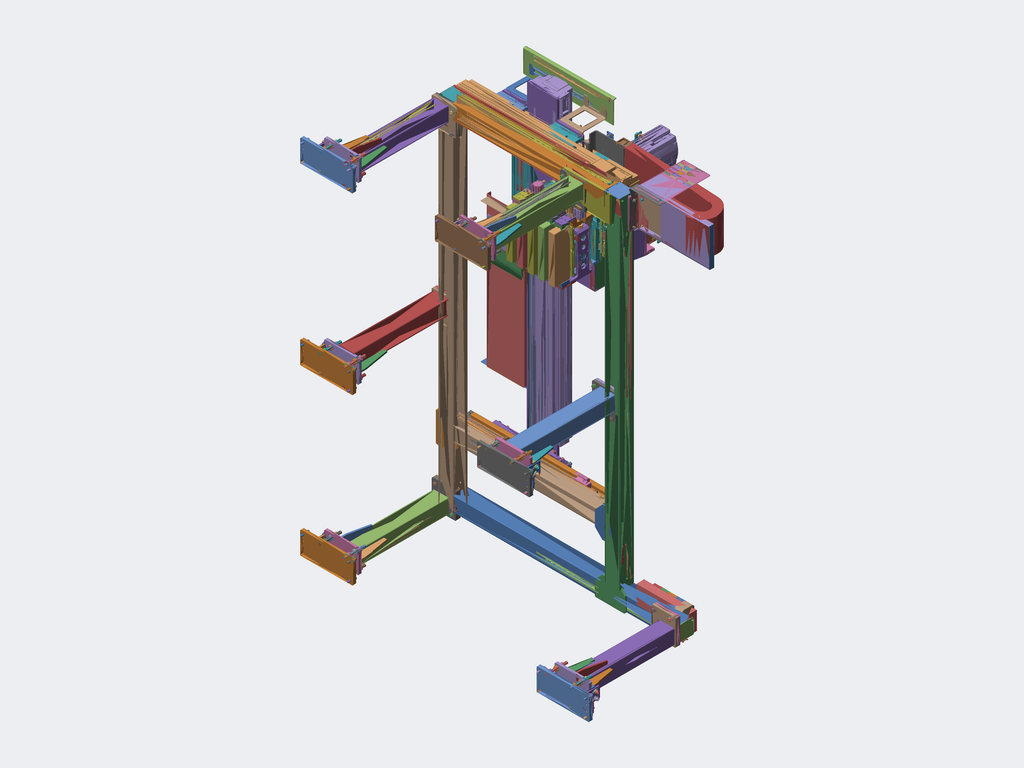Assembly | STEP file | 3599 different items | 3599 placed
Parts list (item | name | quantity | parent item | size | volume), first 284 of 3599 items:
1 | [LR-XN11P]-Part-1 | x1 | in [LR-XN11P] | 12.6 x 34.5 x 105.605 mm | 23912 mm3
2 | [LR-XN11P]-Part-2 | x1 | in [LR-XN11P] | 2.25 x 17.6 x 14.4 mm | 152.141 mm3
3 | [LR-XN12P]-Part-1 | x1 | in [LR-XN12P] | 14.78 x 34.5 x 105.605 mm | 23972 mm3
4 | [LR-XN12P]-Part-2 | x1 | in [LR-XN12P] | 2.25 x 17.6 x 14.4 mm | 152.141 mm3
5 | [LR-XN12P]-Part-1-1 | x1 | in [LR-XN12P]-1 | 14.78 x 34.5 x 105.605 mm | 23972 mm3
6 | [LR-XN12P]-Part-2-1 | x1 | in [LR-XN12P]-1 | 2.25 x 17.6 x 14.4 mm | 152.141 mm3
7 | [LR-XN12P]-Part-1-2 | x1 | in [LR-XN12P]-2 | 14.78 x 34.5 x 105.605 mm | 23972 mm3
8 | [LR-XN12P]-Part-2-2 | x1 | in [LR-XN12P]-2 | 2.25 x 17.6 x 14.4 mm | 152.141 mm3
9 | [LR-XN12P]-Part-1-3 | x1 | in [LR-XN12P]-3 | 14.78 x 34.5 x 105.605 mm | 23972 mm3
10 | [LR-XN12P]-Part-2-3 | x1 | in [LR-XN12P]-3 | 2.25 x 17.6 x 14.4 mm | 152.141 mm3
11 | [OP-26751]-Part-1 | x1 | in [OP-26751] | 6 x 53.8 x 20.8 mm | 4707 mm3
12 | [OP-26751]-Part-2 | x1 | in [OP-26751] | 6 x 53.8 x 20.8 mm | 4707 mm3
13 | SANBN6-25-Part-1 | x1 | in SANBN6-25 | 25 x 6 x 6 mm | 665.544 mm3
14 | SANBN6-25-Part-2 | x1 | in SANBN6-25 | 4 x 10 x 11.5 mm | 231.302 mm3
15 | SANBN6-25-Part-1-1 | x1 | in SANBN6-25-1 | 25 x 6 x 6 mm | 665.544 mm3
16 | SANBN6-25-Part-2-1 | x1 | in SANBN6-25-1 | 4 x 10 x 11.5 mm | 231.302 mm3
17 | SANBN6-25-Part-1-2 | x1 | in SANBN6-25-2 | 25 x 6 x 6 mm | 665.544 mm3
18 | SANBN6-25-Part-2-2 | x1 | in SANBN6-25-2 | 4 x 10 x 11.5 mm | 231.302 mm3
19 | SANBN6-25-Part-1-3 | x1 | in SANBN6-25-3 | 25 x 6 x 6 mm | 665.544 mm3
20 | SANBN6-25-Part-2-3 | x1 | in SANBN6-25-3 | 4 x 10 x 11.5 mm | 231.302 mm3
21 | 25A-CDQ2B40-45DZ-M9BWSDPC-Part-1 | x1 | in 25A-CDQ2B40-45DZ-M9BWSDPC | 84.5 x 52 x 57 mm | 122749 mm3
22 | 25A-CDQ2B40-45DZ-M9BWSDPC-Part-2 | x1 | in 25A-CDQ2B40-45DZ-M9BWSDPC | 27 x 4 x 4.6 mm | 354.995 mm3
23 | 25A-CDQ2B40-45DZ-M9BWSDPC-Part-3 | x1 | in 25A-CDQ2B40-45DZ-M9BWSDPC | 27 x 4 x 4.6 mm | 354.995 mm3
24 | 25A-CDQ2B40-45DZ-M9BWSDPC-Part-1-1 | x1 | in 25A-CDQ2B40-45DZ-M9BWSDPC-1 | 27 x 4 x 4.6 mm | 354.995 mm3
25 | 25A-CDQ2B40-45DZ-M9BWSDPC-Part-2-1 | x1 | in 25A-CDQ2B40-45DZ-M9BWSDPC-1 | 27 x 4 x 4.6 mm | 354.995 mm3
26 | 25A-CDQ2B40-45DZ-M9BWSDPC-Part-3-1 | x1 | in 25A-CDQ2B40-45DZ-M9BWSDPC-1 | 84.5 x 52 x 57 mm | 122749 mm3
27 | J454-EBZ05-98-04-Part-1 | x1 | in J454-EBZ05-98-04 | 380 x 13 x 15 mm | 62425 mm3
28 | J454-EBZ05-98-04-Part-1-1 | x1 | in J454-EBZ05-98-04-1 | 380 x 13 x 15 mm | 62425 mm3
29 | AS2201FG-01-06S | x1 | in Unit 4 purchased part 1 | 14.2 x 35.2 x 27.5 mm | 4200 mm3
30 | AS2201FG-01-06S-1 | x1 | in Unit 4 purchased part 1 | 14.2 x 35.2 x 27.5 mm | 4200 mm3
31 | AS2201FG-01-06S-2 | x1 | in Unit 4 purchased part 1 | 14.2 x 35.2 x 27.5 mm | 4200 mm3
32 | AS2201FG-01-06S-3 | x1 | in Unit 4 purchased part 1 | 14.2 x 35.2 x 27.5 mm | 4200 mm3
33 | AS2002FG-06A | x1 | in Unit 4 purchased part 1 | 12.3 x 31.4 x 43.1 mm | 6190 mm3
34 | AS2002FG-06A-1 | x1 | in Unit 4 purchased part 1 | 12.3 x 31.4 x 43.1 mm | 6190 mm3
35 | AS2002FG-06A-2 | x1 | in Unit 4 purchased part 1 | 12.3 x 31.4 x 43.1 mm | 6190 mm3
36 | AS2002FG-06A-3 | x1 | in Unit 4 purchased part 1 | 12.3 x 31.4 x 43.1 mm | 6190 mm3
37 | AS2002FG-06A-4 | x1 | in Unit 4 purchased part 1 | 12.3 x 31.4 x 43.1 mm | 6190 mm3
38 | AS2002FG-06A-5 | x1 | in Unit 4 purchased part 1 | 12.3 x 31.4 x 43.1 mm | 6190 mm3
39 | AS2002FG-06A-6 | x1 | in Unit 4 purchased part 1 | 12.3 x 31.4 x 43.1 mm | 6190 mm3
40 | AS2002FG-06A-7 | x1 | in Unit 4 purchased part 1 | 12.3 x 31.4 x 43.1 mm | 6190 mm3
41 | AS2002FG-06A-8 | x1 | in Unit 4 purchased part 1 | 12.3 x 31.4 x 43.1 mm | 6190 mm3
42 | AS2002FG-06A-9 | x1 | in Unit 4 purchased part 1 | 12.3 x 31.4 x 43.1 mm | 6190 mm3
43 | BB62-M3-30L | x1 | in Unit 4 purchased part 1 | 5.5 x 33 x 5.5 mm | 272.045 mm3
44 | BB62-M3-30L-1 | x1 | in Unit 4 purchased part 1 | 5.5 x 33 x 5.5 mm | 272.045 mm3
45 | BB62-M3-30L-2 | x1 | in Unit 4 purchased part 1 | 5.5 x 33 x 5.5 mm | 272.045 mm3
46 | BB62-M3-30L-3 | x1 | in Unit 4 purchased part 1 | 5.5 x 33 x 5.5 mm | 272.045 mm3
47 | BB62-M3-30L-4 | x1 | in Unit 4 purchased part 1 | 5.5 x 33 x 5.5 mm | 272.045 mm3
48 | BB62-M3-30L-5 | x1 | in Unit 4 purchased part 1 | 5.5 x 33 x 5.5 mm | 272.045 mm3
49 | BB62-M3-30L-6 | x1 | in Unit 4 purchased part 1 | 5.5 x 33 x 5.5 mm | 272.045 mm3
50 | BB62-M3-30L-7 | x1 | in Unit 4 purchased part 1 | 5.5 x 33 x 5.5 mm | 272.045 mm3
51 | J454-EBZ05-06-00-Part-1 | x1 | in J454-EBZ05-06-00 | 406 x 216 x 12.5 mm | 586432 mm3
52 | BB62-M5-12L | x1 | in J454-EBZ05-06-00 | 8.5 x 17 x 8.5 mm | 467.118 mm3
53 | BB62-M5-12L-1 | x1 | in J454-EBZ05-06-00 | 8.5 x 17 x 8.5 mm | 467.118 mm3
54 | BB62-M5-12L-2 | x1 | in J454-EBZ05-06-00 | 8.5 x 17 x 8.5 mm | 467.118 mm3
55 | BB62-M5-12L-3 | x1 | in J454-EBZ05-06-00 | 8.5 x 17 x 8.5 mm | 467.118 mm3
56 | BB62-M5-12L-4 | x1 | in J454-EBZ05-06-00 | 8.5 x 17 x 8.5 mm | 467.118 mm3
57 | BB62-M5-12L-5 | x1 | in J454-EBZ05-06-00 | 8.5 x 17 x 8.5 mm | 467.118 mm3
58 | BB62-M5-12L-6 | x1 | in J454-EBZ05-06-00 | 8.5 x 17 x 8.5 mm | 467.118 mm3
59 | BB62-M5-12L-7 | x1 | in J454-EBZ05-06-00 | 8.5 x 17 x 8.5 mm | 467.118 mm3
60 | ZZ21-M5 | x1 | in J454-EBZ05-06-00 | 12 x 0.8 x 12 mm | 71.471 mm3
61 | ZZ24-M5 | x1 | in J454-EBZ05-06-00 | 9.2 x 1.3 x 9.188 mm | 56.371 mm3
62 | BB62-M5-20L | x1 | in J454-EBZ05-06-00 | 8.5 x 25 x 8.5 mm | 624.198 mm3
63 | ZZ24-M5-1 | x1 | in J454-EBZ05-06-00 | 9.2 x 1.3 x 9.188 mm | 56.371 mm3
64 | ZZ21-M5-1 | x1 | in J454-EBZ05-06-00 | 12 x 0.8 x 12 mm | 71.471 mm3
65 | BB62-M5-20L-1 | x1 | in J454-EBZ05-06-00 | 8.5 x 25 x 8.5 mm | 624.198 mm3
66 | ZZ24-M5-2 | x1 | in J454-EBZ05-06-00 | 9.2 x 1.3 x 9.188 mm | 56.371 mm3
67 | ZZ21-M5-2 | x1 | in J454-EBZ05-06-00 | 12 x 0.8 x 12 mm | 71.471 mm3
68 | BB62-M5-20L-2 | x1 | in J454-EBZ05-06-00 | 8.5 x 25 x 8.5 mm | 624.198 mm3
69 | ZZ24-M5-3 | x1 | in J454-EBZ05-06-00 | 9.2 x 1.3 x 9.188 mm | 56.371 mm3
70 | ZZ21-M5-3 | x1 | in J454-EBZ05-06-00 | 12 x 0.8 x 12 mm | 71.471 mm3
71 | BB62-M5-20L-3 | x1 | in J454-EBZ05-06-00 | 8.5 x 25 x 8.5 mm | 624.198 mm3
72 | ZZ24-M5-4 | x1 | in J454-EBZ05-06-00 | 9.2 x 1.3 x 9.188 mm | 56.371 mm3
73 | ZZ21-M5-4 | x1 | in J454-EBZ05-06-00 | 12 x 0.8 x 12 mm | 71.471 mm3
74 | BB62-M5-20L-4 | x1 | in J454-EBZ05-06-00 | 8.5 x 25 x 8.5 mm | 624.198 mm3
75 | ZZ24-M5-5 | x1 | in J454-EBZ05-06-00 | 9.2 x 1.3 x 9.188 mm | 56.371 mm3
76 | ZZ21-M5-5 | x1 | in J454-EBZ05-06-00 | 12 x 0.8 x 12 mm | 71.471 mm3
77 | BB62-M5-20L-5 | x1 | in J454-EBZ05-06-00 | 8.5 x 25 x 8.5 mm | 624.198 mm3
78 | J454-EBZ05-07-00-Part-1 | x1 | in J454-EBZ05-07-00 | 74 x 66 x 38 mm | 56161 mm3
79 | MSTMS8-20 | x1 | in J454-EBZ05-07-00 | 20 x 8 x 7.85 mm | 827.27 mm3
80 | MSTMS8-20-1 | x1 | in J454-EBZ05-07-00 | 20 x 8 x 7.85 mm | 827.27 mm3
81 | BB62-M8-30L | x1 | in J454-EBZ05-07-00 | 13 x 38 x 13 mm | 2381 mm3
82 | BB62-M8-30L-1 | x1 | in J454-EBZ05-07-00 | 13 x 38 x 13 mm | 2381 mm3
83 | ZZ21-M8 | x1 | in J454-EBZ05-07-00 | 18 x 1.6 x 18 mm | 316.358 mm3
84 | ZZ24-M8 | x1 | in J454-EBZ05-07-00 | 15.4 x 2 x 15.4 mm | 263.048 mm3
85 | ZZ21-M8-1 | x1 | in J454-EBZ05-07-00 | 18 x 1.6 x 18 mm | 316.358 mm3
86 | ZZ24-M8-1 | x1 | in J454-EBZ05-07-00 | 15.4 x 2 x 15.4 mm | 263.048 mm3
87 | BB62-M5-90L | x1 | in J454-EBZ05-07-00 | 8.5 x 95 x 8.5 mm | 2008 mm3
88 | BB62-M5-90L-1 | x1 | in J454-EBZ05-07-00 | 8.5 x 95 x 8.5 mm | 2008 mm3
89 | BB62-M5-90L-2 | x1 | in J454-EBZ05-07-00 | 8.5 x 95 x 8.5 mm | 2008 mm3
90 | BB62-M5-90L-3 | x1 | in J454-EBZ05-07-00 | 8.5 x 95 x 8.5 mm | 2008 mm3
91 | J454-EBZ05-05-00-Part-1 | x1 | in J454-EBZ05-05-00 | 180 x 30 x 15 mm | 71858 mm3
92 | MSTMS8-20-2 | x1 | in J454-EBZ05-05-00 | 20 x 8 x 7.85 mm | 856.572 mm3
93 | J454-EBZ05-01-04-Part-1 | x1 | in J454-EBZ05-01-04 | 448 x 200 x 12 mm | 706268 mm3
94 | ZZ21-M8-2 | x1 | in J454-EBZ05-01-04 | 18 x 1.6 x 18 mm | 316.358 mm3
95 | ZZ24-M8-2 | x1 | in J454-EBZ05-01-04 | 15.4 x 2 x 15.383 mm | 252.413 mm3
96 | BB62-M8-65L | x1 | in J454-EBZ05-01-04 | 13 x 73 x 13 mm | 4140 mm3
97 | ZZ24-M8-3 | x1 | in J454-EBZ05-01-04 | 15.4 x 2 x 15.383 mm | 252.413 mm3
98 | ZZ21-M8-3 | x1 | in J454-EBZ05-01-04 | 18 x 1.6 x 18 mm | 316.358 mm3
99 | BB62-M8-65L-1 | x1 | in J454-EBZ05-01-04 | 13 x 73 x 13 mm | 4140 mm3
100 | ZZ24-M8-4 | x1 | in J454-EBZ05-01-04 | 15.4 x 2 x 15.383 mm | 252.413 mm3
101 | ZZ21-M8-4 | x1 | in J454-EBZ05-01-04 | 18 x 1.6 x 18 mm | 316.358 mm3
102 | BB62-M8-65L-2 | x1 | in J454-EBZ05-01-04 | 13 x 73 x 13 mm | 4140 mm3
103 | ZZ24-M8-5 | x1 | in J454-EBZ05-01-04 | 15.4 x 2 x 15.383 mm | 252.413 mm3
104 | ZZ21-M8-5 | x1 | in J454-EBZ05-01-04 | 18 x 1.6 x 18 mm | 316.358 mm3
105 | BB62-M8-65L-3 | x1 | in J454-EBZ05-01-04 | 13 x 73 x 13 mm | 4140 mm3
106 | ZZ24-M8-6 | x1 | in J454-EBZ05-01-04 | 15.4 x 2 x 15.383 mm | 252.413 mm3
107 | ZZ21-M8-6 | x1 | in J454-EBZ05-01-04 | 18 x 1.6 x 18 mm | 316.358 mm3
108 | BB62-M8-65L-4 | x1 | in J454-EBZ05-01-04 | 13 x 73 x 13 mm | 4140 mm3
109 | ZZ24-M8-7 | x1 | in J454-EBZ05-01-04 | 15.4 x 2 x 15.383 mm | 252.413 mm3
110 | ZZ21-M8-7 | x1 | in J454-EBZ05-01-04 | 18 x 1.6 x 18 mm | 316.358 mm3
111 | BB62-M8-65L-5 | x1 | in J454-EBZ05-01-04 | 13 x 73 x 13 mm | 4140 mm3
112 | ZZ24-M8-8 | x1 | in J454-EBZ05-01-04 | 15.4 x 2 x 15.383 mm | 252.413 mm3
113 | ZZ21-M8-8 | x1 | in J454-EBZ05-01-04 | 18 x 1.6 x 18 mm | 316.358 mm3
114 | BB62-M8-65L-6 | x1 | in J454-EBZ05-01-04 | 13 x 73 x 13 mm | 4140 mm3
115 | ZZ24-M8-9 | x1 | in J454-EBZ05-01-04 | 15.4 x 2 x 15.383 mm | 252.413 mm3
116 | ZZ21-M8-9 | x1 | in J454-EBZ05-01-04 | 18 x 1.6 x 18 mm | 316.358 mm3
117 | BB62-M8-65L-7 | x1 | in J454-EBZ05-01-04 | 13 x 73 x 13 mm | 4140 mm3
118 | MSTMS8-20-3 | x1 | in J454-EBZ05-01-04 | 20 x 8 x 7.85 mm | 856.572 mm3
119 | MSTMS8-20-4 | x1 | in J454-EBZ05-01-04 | 20 x 8 x 7.85 mm | 856.572 mm3
120 | BB62-M6-15L | x1 | in J454-EBZ05-01-04 | 10 x 21 x 10 mm | 798.222 mm3
121 | BB62-M6-15L-1 | x1 | in J454-EBZ05-01-04 | 10 x 21 x 10 mm | 798.222 mm3
122 | BB62-M6-15L-2 | x1 | in J454-EBZ05-01-04 | 10 x 21 x 10 mm | 798.222 mm3
123 | BB62-M6-15L-3 | x1 | in J454-EBZ05-01-04 | 10 x 21 x 10 mm | 798.222 mm3
124 | BB62-M6-15L-4 | x1 | in J454-EBZ05-01-04 | 10 x 21 x 10 mm | 798.222 mm3
125 | BB62-M6-15L-5 | x1 | in J454-EBZ05-01-04 | 10 x 21 x 10 mm | 798.222 mm3
126 | BB62-M6-15L-6 | x1 | in J454-EBZ05-01-04 | 10 x 21 x 10 mm | 798.222 mm3
127 | BB62-M6-15L-7 | x1 | in J454-EBZ05-01-04 | 10 x 21 x 10 mm | 798.222 mm3
128 | BB62-M6-15L-8 | x1 | in J454-EBZ05-01-04 | 10 x 21 x 10 mm | 798.222 mm3
129 | BB62-M6-15L-9 | x1 | in J454-EBZ05-01-04 | 10 x 21 x 10 mm | 798.222 mm3
130 | BB62-M6-15L-10 | x1 | in J454-EBZ05-01-04 | 10 x 21 x 10 mm | 798.222 mm3
131 | BB62-M6-15L-11 | x1 | in J454-EBZ05-01-04 | 10 x 21 x 10 mm | 798.222 mm3
132 | MRB-85 | x1 | in J454-EBZ05-01-04 | 85 x 35 x 7.3 mm | 5359 mm3
133 | WSX-SUS-M4X10-1.5 | x1 | in J454-EBZ05-01-04 | 10 x 1.5 x 10 mm | 93.953 mm3
134 | BB62-M4-12L | x1 | in J454-EBZ05-01-04 | 7 x 16 x 7 mm | 280.182 mm3
135 | WSX-SUS-M4X10-1.5-1 | x1 | in J454-EBZ05-01-04 | 10 x 1.5 x 10 mm | 93.953 mm3
136 | BB62-M4-12L-1 | x1 | in J454-EBZ05-01-04 | 7 x 16 x 7 mm | 280.182 mm3
137 | J454-EBZ05-02-00-Part-1 | x1 | in J454-EBZ05-02-00 | 200 x 174 x 12 mm | 291304 mm3
138 | MSTMS8-20-5 | x1 | in J454-EBZ05-02-00 | 20 x 8 x 7.85 mm | 856.572 mm3
139 | MSTMS8-20-6 | x1 | in J454-EBZ05-02-00 | 20 x 8 x 7.85 mm | 856.572 mm3
140 | BB62-M6-15L-12 | x1 | in J454-EBZ05-02-00 | 10 x 21 x 10 mm | 798.222 mm3
141 | BB62-M6-15L-13 | x1 | in J454-EBZ05-02-00 | 10 x 21 x 10 mm | 798.222 mm3
142 | BB62-M6-15L-14 | x1 | in J454-EBZ05-02-00 | 10 x 21 x 10 mm | 798.222 mm3
143 | BB62-M6-15L-15 | x1 | in J454-EBZ05-02-00 | 10 x 21 x 10 mm | 798.222 mm3
144 | BB62-M6-15L-16 | x1 | in J454-EBZ05-02-00 | 10 x 21 x 10 mm | 798.222 mm3
145 | BB62-M6-15L-17 | x1 | in J454-EBZ05-02-00 | 10 x 21 x 10 mm | 798.222 mm3
146 | BB62-M6-15L-18 | x1 | in J454-EBZ05-02-00 | 10 x 21 x 10 mm | 798.222 mm3
147 | BB62-M6-15L-19 | x1 | in J454-EBZ05-02-00 | 10 x 21 x 10 mm | 798.222 mm3
148 | BB62-M6-15L-20 | x1 | in J454-EBZ05-02-00 | 10 x 21 x 10 mm | 798.222 mm3
149 | BB62-M6-15L-21 | x1 | in J454-EBZ05-02-00 | 10 x 21 x 10 mm | 798.222 mm3
150 | MSTMS8-20-7 | x1 | in J454-EBZ05-02-00 | 20 x 8 x 7.85 mm | 856.572 mm3
151 | MSTMS8-20-8 | x1 | in J454-EBZ05-02-00 | 20 x 8 x 7.85 mm | 856.572 mm3
152 | ZZ24-M10 | x1 | in J454-EBZ05-02-00 | 18.4 x 2.5 x 18.378 mm | 434.673 mm3
153 | ZZ24-M10-1 | x1 | in J454-EBZ05-02-00 | 18.4 x 2.5 x 18.378 mm | 434.673 mm3
154 | ZZ24-M10-2 | x1 | in J454-EBZ05-02-00 | 18.4 x 2.5 x 18.378 mm | 434.673 mm3
155 | ZZ24-M10-3 | x1 | in J454-EBZ05-02-00 | 18.4 x 2.5 x 18.378 mm | 434.673 mm3
156 | ZZ24-M10-4 | x1 | in J454-EBZ05-02-00 | 18.4 x 2.5 x 18.378 mm | 434.673 mm3
157 | ZZ24-M10-5 | x1 | in J454-EBZ05-02-00 | 18.4 x 2.5 x 18.378 mm | 434.673 mm3
158 | WSSS20-10-4 | x1 | in J454-EBZ05-02-00 | 4 x 20 x 20 mm | 918.916 mm3
159 | BB62-M10-30L | x1 | in J454-EBZ05-02-00 | 16 x 40 x 16 mm | 3957 mm3
160 | WSSS20-10-4-1 | x1 | in J454-EBZ05-02-00 | 4 x 20 x 20 mm | 918.916 mm3
161 | BB62-M10-30L-1 | x1 | in J454-EBZ05-02-00 | 16 x 40 x 16 mm | 3957 mm3
162 | WSSS20-10-4-2 | x1 | in J454-EBZ05-02-00 | 4 x 20 x 20 mm | 918.916 mm3
163 | BB62-M10-30L-2 | x1 | in J454-EBZ05-02-00 | 16 x 40 x 16 mm | 3957 mm3
164 | WSSS20-10-4-3 | x1 | in J454-EBZ05-02-00 | 4 x 20 x 20 mm | 918.916 mm3
165 | BB62-M10-30L-3 | x1 | in J454-EBZ05-02-00 | 16 x 40 x 16 mm | 3957 mm3
166 | WSSS20-10-4-4 | x1 | in J454-EBZ05-02-00 | 4 x 20 x 20 mm | 918.916 mm3
167 | BB62-M10-30L-4 | x1 | in J454-EBZ05-02-00 | 16 x 40 x 16 mm | 3957 mm3
168 | WSSS20-10-4-5 | x1 | in J454-EBZ05-02-00 | 4 x 20 x 20 mm | 918.916 mm3
169 | BB62-M10-30L-5 | x1 | in J454-EBZ05-02-00 | 16 x 40 x 16 mm | 3957 mm3
170 | J454-EBZ05-04-00-Part-1 | x1 | in J454-EBZ05-04-00 | 87 x 96 x 12 mm | 74063 mm3
171 | ZZ21-M6 | x1 | in J454-EBZ05-04-00 | 13 x 1 x 13 mm | 99.549 mm3
172 | ZZ24-M6 | x1 | in J454-EBZ05-04-00 | 12.2 x 1.5 x 12.188 mm | 124.605 mm3
173 | BB62-M6-25L | x1 | in J454-EBZ05-04-00 | 10 x 31 x 10 mm | 1081 mm3
174 | ZZ24-M6-1 | x1 | in J454-EBZ05-04-00 | 12.2 x 1.5 x 12.188 mm | 124.605 mm3
175 | ZZ21-M6-1 | x1 | in J454-EBZ05-04-00 | 13 x 1 x 13 mm | 99.549 mm3
176 | BB62-M6-25L-1 | x1 | in J454-EBZ05-04-00 | 10 x 31 x 10 mm | 1081 mm3
177 | ZZ24-M6-2 | x1 | in J454-EBZ05-04-00 | 12.2 x 1.5 x 12.188 mm | 124.605 mm3
178 | ZZ21-M6-2 | x1 | in J454-EBZ05-04-00 | 13 x 1 x 13 mm | 99.549 mm3
179 | BB62-M6-25L-2 | x1 | in J454-EBZ05-04-00 | 10 x 31 x 10 mm | 1081 mm3
180 | ZZ24-M6-3 | x1 | in J454-EBZ05-04-00 | 12.2 x 1.5 x 12.188 mm | 124.605 mm3
181 | ZZ21-M6-3 | x1 | in J454-EBZ05-04-00 | 13 x 1 x 13 mm | 99.549 mm3
182 | BB62-M6-25L-3 | x1 | in J454-EBZ05-04-00 | 10 x 31 x 10 mm | 1081 mm3
183 | J454-EBZ05-08-00-Part-1 | x1 | in J454-EBZ05-08-00 | 75 x 92 x 16 mm | 52479 mm3
184 | BB62-M5-90L-4 | x1 | in J454-EBZ05-08-00 | 8.5 x 95 x 8.5 mm | 2008 mm3
185 | BB62-M5-90L-5 | x1 | in J454-EBZ05-08-00 | 8.5 x 95 x 8.5 mm | 2008 mm3
186 | BB62-M5-90L-6 | x1 | in J454-EBZ05-08-00 | 8.5 x 95 x 8.5 mm | 2008 mm3
187 | BB62-M5-90L-7 | x1 | in J454-EBZ05-08-00 | 8.5 x 95 x 8.5 mm | 2008 mm3
188 | MSTMS8-20-9 | x1 | in J454-EBZ05-08-00 | 20 x 8 x 7.85 mm | 827.27 mm3
189 | MSTMS8-20-10 | x1 | in J454-EBZ05-08-00 | 20 x 8 x 7.85 mm | 827.27 mm3
190 | ZZ21-M8-10 | x1 | in J454-EBZ05-08-00 | 18 x 1.6 x 18 mm | 316.358 mm3
191 | ZZ21-M8-11 | x1 | in J454-EBZ05-08-00 | 18 x 1.6 x 18 mm | 316.358 mm3
192 | ZZ24-M8-10 | x1 | in J454-EBZ05-08-00 | 15.4 x 2 x 15.383 mm | 252.413 mm3
193 | ZZ24-M8-11 | x1 | in J454-EBZ05-08-00 | 15.4 x 2 x 15.383 mm | 252.413 mm3
194 | BB62-M8-30L-2 | x1 | in J454-EBZ05-08-00 | 13 x 38 x 13 mm | 2381 mm3
195 | BB62-M8-30L-3 | x1 | in J454-EBZ05-08-00 | 13 x 38 x 13 mm | 2381 mm3
196 | J454-EBZ05-09-00-Part-1 | x1 | in J454-EBZ05-09-00 | 13 x 42 x 16 mm | 7348 mm3
197 | ZZ21-M6-4 | x1 | in J454-EBZ05-09-00 | 13 x 1 x 13 mm | 99.549 mm3
198 | ZZ21-M6-5 | x1 | in J454-EBZ05-09-00 | 13 x 1 x 13 mm | 99.549 mm3
199 | ZZ24-M6-4 | x1 | in J454-EBZ05-09-00 | 12.2 x 1.5 x 12.188 mm | 124.605 mm3
200 | ZZ24-M6-5 | x1 | in J454-EBZ05-09-00 | 12.2 x 1.5 x 12.188 mm | 124.605 mm3
201 | BB62-M6-25L-4 | x1 | in J454-EBZ05-09-00 | 10 x 31 x 10 mm | 1081 mm3
202 | BB62-M6-25L-5 | x1 | in J454-EBZ05-09-00 | 10 x 31 x 10 mm | 1081 mm3
203 | J454-EBZ05-09-00-Part-1-1 | x1 | in J454-EBZ05-09-00-1 | 13 x 42 x 16 mm | 7348 mm3
204 | ZZ21-M6-6 | x1 | in J454-EBZ05-09-00-1 | 13 x 1 x 13 mm | 99.549 mm3
205 | ZZ21-M6-7 | x1 | in J454-EBZ05-09-00-1 | 13 x 1 x 13 mm | 99.549 mm3
206 | ZZ24-M6-6 | x1 | in J454-EBZ05-09-00-1 | 12.2 x 1.5 x 12.188 mm | 124.605 mm3
207 | ZZ24-M6-7 | x1 | in J454-EBZ05-09-00-1 | 12.2 x 1.5 x 12.188 mm | 124.605 mm3
208 | BB62-M6-25L-6 | x1 | in J454-EBZ05-09-00-1 | 10 x 31 x 10 mm | 1081 mm3
209 | BB62-M6-25L-7 | x1 | in J454-EBZ05-09-00-1 | 10 x 31 x 10 mm | 1081 mm3
210 | J454-EBZ05-09-00-Part-1-2 | x1 | in J454-EBZ05-09-00-2 | 13 x 42 x 16 mm | 7348 mm3
211 | ZZ21-M6-8 | x1 | in J454-EBZ05-09-00-2 | 13 x 1 x 13 mm | 99.549 mm3
212 | ZZ21-M6-9 | x1 | in J454-EBZ05-09-00-2 | 13 x 1 x 13 mm | 99.549 mm3
213 | ZZ24-M6-8 | x1 | in J454-EBZ05-09-00-2 | 12.2 x 1.5 x 12.188 mm | 124.605 mm3
214 | ZZ24-M6-9 | x1 | in J454-EBZ05-09-00-2 | 12.2 x 1.5 x 12.188 mm | 124.605 mm3
215 | BB62-M6-25L-8 | x1 | in J454-EBZ05-09-00-2 | 10 x 31 x 10 mm | 1081 mm3
216 | BB62-M6-25L-9 | x1 | in J454-EBZ05-09-00-2 | 10 x 31 x 10 mm | 1081 mm3
217 | J454-EBZ05-09-00-Part-1-3 | x1 | in J454-EBZ05-09-00-3 | 13 x 42 x 16 mm | 7348 mm3
218 | ZZ21-M6-10 | x1 | in J454-EBZ05-09-00-3 | 13 x 1 x 13 mm | 99.549 mm3
219 | ZZ21-M6-11 | x1 | in J454-EBZ05-09-00-3 | 13 x 1 x 13 mm | 99.549 mm3
220 | ZZ24-M6-10 | x1 | in J454-EBZ05-09-00-3 | 12.2 x 1.5 x 12.188 mm | 124.605 mm3
221 | ZZ24-M6-11 | x1 | in J454-EBZ05-09-00-3 | 12.2 x 1.5 x 12.188 mm | 124.605 mm3
222 | BB62-M6-25L-10 | x1 | in J454-EBZ05-09-00-3 | 10 x 31 x 10 mm | 1081 mm3
223 | BB62-M6-25L-11 | x1 | in J454-EBZ05-09-00-3 | 10 x 31 x 10 mm | 1081 mm3
224 | J454-EBZ05-05-00-Part-1-1 | x1 | in J454-EBZ05-05-00-1 | 180 x 30 x 15 mm | 71858 mm3
225 | MSTMS8-20-11 | x1 | in J454-EBZ05-05-00-1 | 20 x 8 x 7.85 mm | 856.572 mm3
226 | J454-EBZ05-32-03 | x1 | in 01_Fixed part | 448 x 120 x 12 mm | 376287 mm3
227 | J454-EBZ05-32-03-1 | x1 | in 01_Fixed part | 448 x 120 x 12 mm | 376287 mm3
228 | 25A-CDQ2B32-15DZ-M9BWSDPC-Part-1 | x1 | in 25A-CDQ2B32-15DZ-M9BWSDPC | 27 x 4 x 4.6 mm | 354.995 mm3
229 | 25A-CDQ2B32-15DZ-M9BWSDPC-Part-2 | x1 | in 25A-CDQ2B32-15DZ-M9BWSDPC | 48 x 45 x 49.5 mm | 58108 mm3
230 | 25A-CDQ2B32-15DZ-M9BWSDPC-Part-3 | x1 | in 25A-CDQ2B32-15DZ-M9BWSDPC | 27 x 4 x 4.6 mm | 354.995 mm3
231 | Rod | x1 | in 25A-CDQ2B32-15DZ-M9BWSDPC | 37 x 32 x 32 mm | 9768 mm3
232 | J454-EBZ05-99-04-Part-1 | x1 | in J454-EBZ05-99-04 | 140 x 16.5 x 20 mm | 40392 mm3
233 | FUF25-70-A | x1 | in Unit 4 purchased part 2-1 | 50 x 25 x 25 mm | 9148 mm3
234 | FUF25-70-A-1 | x1 | in Unit 4 purchased part 2-1 | 50 x 25 x 25 mm | 9148 mm3
235 | FWSSS-D27-V19-T3 | x1 | in Unit 4 purchased part 2-1 | 27 x 27 x 3 mm | 830.951 mm3
236 | FWSSS-D27-V19-T3-1 | x1 | in Unit 4 purchased part 2-1 | 27 x 27 x 3 mm | 830.951 mm3
237 | KQG2H06-01S | x1 | in Unit 4 purchased part 2-1 | 13.856 x 24.3 x 12 mm | 1839 mm3
238 | KQG2H06-01S-1 | x1 | in Unit 4 purchased part 2-1 | 13.856 x 24.3 x 12 mm | 1839 mm3
239 | BB62-M3-40L | x1 | in Unit 4 purchased part 2-1 | 5.5 x 43 x 5.5 mm | 342.731 mm3
240 | BB62-M3-40L-1 | x1 | in Unit 4 purchased part 2-1 | 5.5 x 43 x 5.5 mm | 342.731 mm3
241 | BB62-M5-50L | x1 | in Unit 4 purchased part 2-1 | 8.5 x 55 x 8.5 mm | 1213 mm3
242 | BB62-M5-50L-1 | x1 | in Unit 4 purchased part 2-1 | 8.5 x 55 x 8.5 mm | 1213 mm3
243 | BB62-M5-50L-2 | x1 | in Unit 4 purchased part 2-1 | 8.5 x 55 x 8.5 mm | 1213 mm3
244 | BB62-M5-50L-3 | x1 | in Unit 4 purchased part 2-1 | 8.5 x 55 x 8.5 mm | 1213 mm3
245 | WSSS12-5-3 | x1 | in Unit 4 purchased part 2-1 | 3 x 12 x 12 mm | 278.251 mm3
246 | WSSS12-5-3-1 | x1 | in Unit 4 purchased part 2-1 | 3 x 12 x 12 mm | 278.251 mm3
247 | WSSS12-5-3-2 | x1 | in Unit 4 purchased part 2-1 | 3 x 12 x 12 mm | 278.251 mm3
248 | WSSS12-5-3-3 | x1 | in Unit 4 purchased part 2-1 | 3 x 12 x 12 mm | 278.251 mm3
249 | J454-EBZ05-17-00-Part-1 | x1 | in J454-EBZ05-17-00 | 19 x 19 x 18 mm | 4103 mm3
250 | BB62-M5-15L | x1 | in J454-EBZ05-17-00 | 8.5 x 20 x 8.5 mm | 526.023 mm3
251 | J454-EBZ05-17-00-Part-1-1 | x1 | in J454-EBZ05-17-00-1 | 19 x 19 x 18 mm | 4103 mm3
252 | BB62-M5-15L-1 | x1 | in J454-EBZ05-17-00-1 | 8.5 x 20 x 8.5 mm | 526.023 mm3
253 | LR-XH50-Part-1 | x1 | in LR-XH50 | 9.4 x 39.451 x 29.153 mm | 4011 mm3
254 | WSX-SUS-M5X12-2 | x1 | in J454-EBZ05-18-00 | 12 x 2 x 12 mm | 178.678 mm3
255 | ZZ24-M5-6 | x1 | in J454-EBZ05-18-00 | 9.2 x 1.3 x 9.188 mm | 56.371 mm3
256 | ZZ24-M5-7 | x1 | in J454-EBZ05-18-00 | 9.2 x 1.3 x 9.188 mm | 56.371 mm3
257 | BB62-M5-22L | x1 | in J454-EBZ05-18-00 | 8.5 x 27 x 8.5 mm | 663.468 mm3
258 | BB62-M5-22L-1 | x1 | in J454-EBZ05-18-00 | 8.5 x 27 x 8.5 mm | 663.468 mm3
259 | BB62-M3-8L | x1 | in J454-EBZ05-18-00 | 5.5 x 11 x 5.5 mm | 116.536 mm3
260 | BB62-M3-8L-1 | x1 | in J454-EBZ05-18-00 | 5.5 x 11 x 5.5 mm | 116.536 mm3
261 | WSX-SUS-M5X12-2-1 | x1 | in J454-EBZ05-18-00 | 12 x 2 x 12 mm | 178.678 mm3
262 | J454-EBZ05-13-00-Part-1 | x1 | in J454-EBZ05-13-00 | 200 x 48 x 50 mm | 172584 mm3
263 | BB62-M6-15L-22 | x1 | in J454-EBZ05-13-00 | 10 x 21 x 10 mm | 798.222 mm3
264 | BB62-M6-15L-23 | x1 | in J454-EBZ05-13-00 | 10 x 21 x 10 mm | 798.222 mm3
265 | BB62-M6-15L-24 | x1 | in J454-EBZ05-13-00 | 10 x 21 x 10 mm | 798.222 mm3
266 | SSTBB6-25-Part-1 | x1 | in SSTBB6-25 | 29 x 11.5 x 10 mm | 987.027 mm3
267 | SSTBB6-25-Part-2 | x1 | in SSTBB6-25 | 5 x 11.5 x 10 mm | 290.522 mm3
268 | SSTBB6-25-Part-1-1 | x1 | in SSTBB6-25-1 | 29 x 11.5 x 10 mm | 987.027 mm3
269 | SSTBB6-25-Part-2-1 | x1 | in SSTBB6-25-1 | 5 x 11.5 x 10 mm | 290.522 mm3
270 | SSTBB6-25-Part-1-2 | x1 | in SSTBB6-25-2 | 29 x 11.5 x 10 mm | 987.027 mm3
271 | SSTBB6-25-Part-2-2 | x1 | in SSTBB6-25-2 | 5 x 11.5 x 10 mm | 290.522 mm3
272 | SSTBB6-25-Part-1-3 | x1 | in SSTBB6-25-3 | 29 x 11.5 x 10 mm | 987.027 mm3
273 | SSTBB6-25-Part-2-3 | x1 | in SSTBB6-25-3 | 5 x 11.5 x 10 mm | 290.522 mm3
274 | J454-EBZ05-11-03-Part-1 | x1 | in J454-EBZ05-11-03 | 290 x 48 x 62 mm | 468483 mm3
275 | MSTMS8-20-12 | x1 | in J454-EBZ05-11-03 | 20 x 8 x 7.85 mm | 856.572 mm3
276 | MSTMS8-20-13 | x1 | in J454-EBZ05-11-03 | 20 x 8 x 7.85 mm | 856.572 mm3
277 | BB62-M6-18L | x1 | in J454-EBZ05-11-03 | 10 x 24 x 10 mm | 883.045 mm3
278 | BB62-M6-18L-1 | x1 | in J454-EBZ05-11-03 | 10 x 24 x 10 mm | 883.045 mm3
279 | BB62-M6-18L-2 | x1 | in J454-EBZ05-11-03 | 10 x 24 x 10 mm | 883.045 mm3
280 | BB62-M6-18L-3 | x1 | in J454-EBZ05-11-03 | 10 x 24 x 10 mm | 883.045 mm3
281 | BB62-M6-18L-4 | x1 | in J454-EBZ05-11-03 | 10 x 24 x 10 mm | 883.045 mm3
282 | BB62-M6-18L-5 | x1 | in J454-EBZ05-11-03 | 10 x 24 x 10 mm | 883.045 mm3
283 | KNCLSS3-8-10 | x1 | in J454-EBZ05-11-03 | 10 x 6 x 6 mm | 210.927 mm3
284 | KNCLSS3-8-10-1 | x1 | in J454-EBZ05-11-03 | 10 x 6 x 6 mm | 210.927 mm3
Placements (level | parent | child | x y z in mm | rotation matrix by rows), first 198 of 3891 lines:
1 | subassembly 2 | J454-EBZ05-00-08 | -0.0 1452.0 1475.0 | 0 0 1 0 1 0 -1 0 0
2 | J454-EBZ05-00-08 | 01_Fixed part | -0.0 -0.0 -0.0 | 1 0 0 0 1 0 0 0 1
3 | 01_Fixed part | Unit 4 purchased part 1 | -0.0 -0.0 -0.0 | 1 0 0 0 1 0 0 0 1
4 | Unit 4 purchased part 1 | [LR-XN11P] | 25.945 113.445 -23.2 | -1 0 0 0 0 1 0 1 0
5 | [LR-XN11P] | [LR-XN11P]-Part-1 | -0.0 -0.0 -0.0 | 1 0 0 0 1 0 0 0 1
5 | [LR-XN11P] | [LR-XN11P]-Part-2 | -0.0 -0.0 -0.0 | 1 0 0 0 1 0 0 0 1
4 | Unit 4 purchased part 1 | [LR-XN12P] | 15.245 113.445 -19.0 | -1 0 0 0 0 1 0 1 0
5 | [LR-XN12P] | [LR-XN12P]-Part-1 | -0.0 -0.0 -0.0 | 1 0 0 0 1 0 0 0 1
5 | [LR-XN12P] | [LR-XN12P]-Part-2 | -0.0 -0.0 -0.0 | 1 0 0 0 1 0 0 0 1
4 | Unit 4 purchased part 1 | [LR-XN12P]-1 | 4.545 113.445 -19.0 | -1 0 0 0 0 1 0 1 0
5 | [LR-XN12P]-1 | [LR-XN12P]-Part-1-1 | -0.0 -0.0 -0.0 | 1 0 0 0 1 0 0 0 1
5 | [LR-XN12P]-1 | [LR-XN12P]-Part-2-1 | -0.0 -0.0 -0.0 | 1 0 0 0 1 0 0 0 1
4 | Unit 4 purchased part 1 | [LR-XN12P]-2 | -6.155 113.445 -19.0 | -1 0 0 0 0 1 0 1 0
5 | [LR-XN12P]-2 | [LR-XN12P]-Part-1-2 | -0.0 -0.0 -0.0 | 1 0 0 0 1 0 0 0 1
5 | [LR-XN12P]-2 | [LR-XN12P]-Part-2-2 | -0.0 -0.0 -0.0 | 1 0 0 0 1 0 0 0 1
4 | Unit 4 purchased part 1 | [LR-XN12P]-3 | -16.855 113.445 -19.0 | -1 0 0 0 0 1 0 1 0
5 | [LR-XN12P]-3 | [LR-XN12P]-Part-1-3 | -0.0 -0.0 -0.0 | 1 0 0 0 1 0 0 0 1
5 | [LR-XN12P]-3 | [LR-XN12P]-Part-2-3 | -0.0 -0.0 -0.0 | 1 0 0 0 1 0 0 0 1
4 | Unit 4 purchased part 1 | [OP-26751] | -37.025 181.9 6.75 | 1 0 0 0 -1 0 0 0 -1
5 | [OP-26751] | [OP-26751]-Part-1 | -0.0 -0.0 -0.0 | 1 0 0 0 1 0 0 0 1
5 | [OP-26751] | [OP-26751]-Part-2 | -0.0 -0.0 -0.0 | 1 0 0 0 1 0 0 0 1
4 | Unit 4 purchased part 1 | SANBN6-25 | -115.0 -16.0 205.0 | 0 -0.5 0.866 0 0.866 0.5 -1 0 0
5 | SANBN6-25 | SANBN6-25-Part-1 | -0.0 -0.0 -0.0 | 1 0 0 0 1 0 0 0 1
5 | SANBN6-25 | SANBN6-25-Part-2 | -0.0 -0.0 -0.0 | 1 0 0 0 1 0 0 0 1
4 | Unit 4 purchased part 1 | SANBN6-25-1 | 115.0 -16.0 205.0 | 0 -0.5 0.866 0 0.866 0.5 -1 0 0
5 | SANBN6-25-1 | SANBN6-25-Part-1-1 | -0.0 -0.0 -0.0 | 1 0 0 0 1 0 0 0 1
5 | SANBN6-25-1 | SANBN6-25-Part-2-1 | -0.0 -0.0 -0.0 | 1 0 0 0 1 0 0 0 1
4 | Unit 4 purchased part 1 | SANBN6-25-2 | 115.0 -16.0 -205.0 | 0 0.5 0.866 0 -0.866 0.5 1 0 0
5 | SANBN6-25-2 | SANBN6-25-Part-1-2 | -0.0 -0.0 -0.0 | 1 0 0 0 1 0 0 0 1
5 | SANBN6-25-2 | SANBN6-25-Part-2-2 | -0.0 -0.0 -0.0 | 1 0 0 0 1 0 0 0 1
4 | Unit 4 purchased part 1 | SANBN6-25-3 | -115.0 -16.0 -205.0 | 0 0.5 0.866 0 -0.866 0.5 1 0 0
5 | SANBN6-25-3 | SANBN6-25-Part-1-3 | -0.0 -0.0 -0.0 | 1 0 0 0 1 0 0 0 1
5 | SANBN6-25-3 | SANBN6-25-Part-2-3 | -0.0 -0.0 -0.0 | 1 0 0 0 1 0 0 0 1
4 | Unit 4 purchased part 1 | 25A-CDQ2B40-45DZ-M9BWSDPC | 26.0 -53.0 -291.5 | 0 0 -1 0 1 0 1 0 0
5 | 25A-CDQ2B40-45DZ-M9BWSDPC | 25A-CDQ2B40-45DZ-M9BWSDPC-Part-1 | -0.0 -0.0 -0.0 | 1 0 0 0 1 0 0 0 1
5 | 25A-CDQ2B40-45DZ-M9BWSDPC | 25A-CDQ2B40-45DZ-M9BWSDPC-Part-2 | -0.0 -0.0 -0.0 | 1 0 0 0 1 0 0 0 1
5 | 25A-CDQ2B40-45DZ-M9BWSDPC | 25A-CDQ2B40-45DZ-M9BWSDPC-Part-3 | -0.0 -0.0 -0.0 | 1 0 0 0 1 0 0 0 1
4 | Unit 4 purchased part 1 | 25A-CDQ2B40-45DZ-M9BWSDPC-1 | -26.0 17.0 31.5 | 0 1 0 0 0 1 1 0 0
5 | 25A-CDQ2B40-45DZ-M9BWSDPC-1 | 25A-CDQ2B40-45DZ-M9BWSDPC-Part-1-1 | -0.0 -0.0 -0.0 | 1 0 0 0 1 0 0 0 1
5 | 25A-CDQ2B40-45DZ-M9BWSDPC-1 | 25A-CDQ2B40-45DZ-M9BWSDPC-Part-2-1 | -0.0 -0.0 -0.0 | 1 0 0 0 1 0 0 0 1
5 | 25A-CDQ2B40-45DZ-M9BWSDPC-1 | 25A-CDQ2B40-45DZ-M9BWSDPC-Part-3-1 | -0.0 -0.0 -0.0 | 1 0 0 0 1 0 0 0 1
4 | Unit 4 purchased part 1 | J454-EBZ05-98-04 | 36.5 -10.0 -195.5 | 0 0 1 0 -1 0 1 0 0
5 | J454-EBZ05-98-04 | J454-EBZ05-98-04-Part-1 | -0.0 -0.0 -0.0 | 1 0 0 0 1 0 0 0 1
4 | Unit 4 purchased part 1 | J454-EBZ05-98-04-1 | -83.5 -10.0 -195.5 | 0 0 1 0 -1 0 1 0 0
5 | J454-EBZ05-98-04-1 | J454-EBZ05-98-04-Part-1-1 | -0.0 -0.0 -0.0 | 1 0 0 0 1 0 0 0 1
4 | Unit 4 purchased part 1 | AS2201FG-01-06S | -30.1 -27.0 -284.0 | 0 -1 0 0 0 1 -1 0 0
4 | Unit 4 purchased part 1 | AS2201FG-01-06S-1 | -30.1 -27.0 -219.5 | 0 -1 0 0 0 1 -1 0 0
4 | Unit 4 purchased part 1 | AS2201FG-01-06S-2 | -0.0 73.1 103.5 | 0 0 -1 0 1 0 1 0 0
4 | Unit 4 purchased part 1 | AS2201FG-01-06S-3 | -0.0 73.1 39.0 | 0 0 -1 0 1 0 1 0 0
4 | Unit 4 purchased part 1 | AS2002FG-06A | -168.45 -24.0 -127.4 | -1 0 0 0 0 -1 0 -1 0
4 | Unit 4 purchased part 1 | AS2002FG-06A-1 | -156.15 -24.0 -127.4 | -1 0 0 0 0 -1 0 -1 0
4 | Unit 4 purchased part 1 | AS2002FG-06A-2 | -168.45 -24.0 -83.6 | -1 0 0 0 0 1 0 1 0
4 | Unit 4 purchased part 1 | AS2002FG-06A-3 | -156.15 -24.0 -83.6 | -1 0 0 0 0 1 0 1 0
4 | Unit 4 purchased part 1 | AS2002FG-06A-4 | -168.45 -24.0 7.1 | -1 0 0 0 0 -1 0 -1 0
4 | Unit 4 purchased part 1 | AS2002FG-06A-5 | -156.15 -24.0 7.1 | -1 0 0 0 0 -1 0 -1 0
4 | Unit 4 purchased part 1 | AS2002FG-06A-6 | -168.45 -24.0 83.6 | -1 0 0 0 0 -1 0 -1 0
4 | Unit 4 purchased part 1 | AS2002FG-06A-7 | -156.15 -24.0 83.6 | -1 0 0 0 0 -1 0 -1 0
4 | Unit 4 purchased part 1 | AS2002FG-06A-8 | -168.45 -24.0 127.4 | -1 0 0 0 0 1 0 1 0
4 | Unit 4 purchased part 1 | AS2002FG-06A-9 | -156.15 -24.0 127.4 | -1 0 0 0 0 1 0 1 0
4 | Unit 4 purchased part 1 | BB62-M3-30L | -174.6 -30.3 134.5 | 0 -1 0 0 0 1 -1 0 0
4 | Unit 4 purchased part 1 | BB62-M3-30L-1 | -174.6 -17.7 134.5 | 0 -1 0 0 0 1 -1 0 0
4 | Unit 4 purchased part 1 | BB62-M3-30L-2 | -174.6 -17.7 76.5 | 0 -1 0 0 0 -1 1 0 0
4 | Unit 4 purchased part 1 | BB62-M3-30L-3 | -174.6 -30.3 76.5 | 0 -1 0 0 0 -1 1 0 0
4 | Unit 4 purchased part 1 | BB62-M3-30L-4 | -174.6 -30.3 -76.5 | 0 -1 0 0 0 1 -1 0 0
4 | Unit 4 purchased part 1 | BB62-M3-30L-5 | -174.6 -17.7 -76.5 | 0 -1 0 0 0 1 -1 0 0
4 | Unit 4 purchased part 1 | BB62-M3-30L-6 | -174.6 -17.7 -134.5 | 0 -1 0 0 0 -1 1 0 0
4 | Unit 4 purchased part 1 | BB62-M3-30L-7 | -174.6 -30.3 -134.5 | 0 -1 0 0 0 -1 1 0 0
3 | 01_Fixed part | J454-EBZ05-06-00 | -0.0 -0.0 -0.0 | 0 1 0 0 0 -1 -1 0 0
4 | J454-EBZ05-06-00 | J454-EBZ05-06-00-Part-1 | -0.0 -0.0 -0.0 | 1 0 0 0 1 0 0 0 1
4 | J454-EBZ05-06-00 | BB62-M5-12L | -0.0 -60.0 6.0 | 0 0 1 -1 0 0 0 -1 0
4 | J454-EBZ05-06-00 | BB62-M5-12L-1 | -0.0 60.0 6.0 | 0 0 1 -1 0 0 0 -1 0
4 | J454-EBZ05-06-00 | BB62-M5-12L-2 | -60.0 -60.0 6.0 | 0 0 1 -1 0 0 0 -1 0
4 | J454-EBZ05-06-00 | BB62-M5-12L-3 | -60.0 60.0 6.0 | 0 0 1 -1 0 0 0 -1 0
4 | J454-EBZ05-06-00 | BB62-M5-12L-4 | 60.0 -60.0 6.0 | 0 0 1 -1 0 0 0 -1 0
4 | J454-EBZ05-06-00 | BB62-M5-12L-5 | 60.0 60.0 6.0 | 0 0 1 -1 0 0 0 -1 0
4 | J454-EBZ05-06-00 | BB62-M5-12L-6 | -120.0 60.0 6.0 | 0 0 1 -1 0 0 0 -1 0
4 | J454-EBZ05-06-00 | BB62-M5-12L-7 | -120.0 -60.0 6.0 | 0 0 1 -1 0 0 0 -1 0
4 | J454-EBZ05-06-00 | ZZ21-M5 | -180.0 -60.0 -0.0 | 0 0 -1 1 0 0 0 -1 0
4 | J454-EBZ05-06-00 | ZZ24-M5 | -180.0 -60.0 -0.8 | 0 0 -1 1 0 0 0 -1 0
4 | J454-EBZ05-06-00 | BB62-M5-20L | -180.0 -60.0 -2.1 | 0 0 -1 1 0 0 0 -1 0
4 | J454-EBZ05-06-00 | ZZ24-M5-1 | 120.0 -60.0 -0.8 | 0 0 -1 1 0 0 0 -1 0
4 | J454-EBZ05-06-00 | ZZ21-M5-1 | 120.0 -60.0 -0.0 | 0 0 -1 1 0 0 0 -1 0
4 | J454-EBZ05-06-00 | BB62-M5-20L-1 | 120.0 -60.0 -2.1 | 0 0 -1 1 0 0 0 -1 0
4 | J454-EBZ05-06-00 | ZZ24-M5-2 | 180.0 -60.0 -0.8 | 0 0 -1 1 0 0 0 -1 0
4 | J454-EBZ05-06-00 | ZZ21-M5-2 | 180.0 -60.0 -0.0 | 0 0 -1 1 0 0 0 -1 0
4 | J454-EBZ05-06-00 | BB62-M5-20L-2 | 180.0 -60.0 -2.1 | 0 0 -1 1 0 0 0 -1 0
4 | J454-EBZ05-06-00 | ZZ24-M5-3 | 180.0 60.0 -0.8 | 0 0 -1 1 0 0 0 -1 0
4 | J454-EBZ05-06-00 | ZZ21-M5-3 | 180.0 60.0 -0.0 | 0 0 -1 1 0 0 0 -1 0
4 | J454-EBZ05-06-00 | BB62-M5-20L-3 | 180.0 60.0 -2.1 | 0 0 -1 1 0 0 0 -1 0
4 | J454-EBZ05-06-00 | ZZ24-M5-4 | 120.0 60.0 -0.8 | 0 0 -1 1 0 0 0 -1 0
4 | J454-EBZ05-06-00 | ZZ21-M5-4 | 120.0 60.0 -0.0 | 0 0 -1 1 0 0 0 -1 0
4 | J454-EBZ05-06-00 | BB62-M5-20L-4 | 120.0 60.0 -2.1 | 0 0 -1 1 0 0 0 -1 0
4 | J454-EBZ05-06-00 | ZZ24-M5-5 | -180.0 60.0 -0.8 | 0 0 -1 1 0 0 0 -1 0
4 | J454-EBZ05-06-00 | ZZ21-M5-5 | -180.0 60.0 0.0 | 0 0 -1 1 0 0 0 -1 0
4 | J454-EBZ05-06-00 | BB62-M5-20L-5 | -180.0 60.0 -2.1 | 0 0 -1 1 0 0 0 -1 0
3 | 01_Fixed part | J454-EBZ05-07-00 | -0.0 12.0 -207.0 | 1 0 0 0 1 0 0 0 1
4 | J454-EBZ05-07-00 | J454-EBZ05-07-00-Part-1 | -0.0 -0.0 -0.0 | 1 0 0 0 1 0 0 0 1
4 | J454-EBZ05-07-00 | MSTMS8-20 | 12.0 -20.0 30.0 | 0 1 0 1 0 0 0 0 -1
4 | J454-EBZ05-07-00 | MSTMS8-20-1 | -12.0 -20.0 30.0 | 0 1 0 1 0 0 0 0 -1
4 | J454-EBZ05-07-00 | BB62-M8-30L | 26.0 3.6 25.0 | 1 0 0 0 1 0 0 0 1
4 | J454-EBZ05-07-00 | BB62-M8-30L-1 | -26.0 3.6 25.0 | 1 0 0 0 1 0 0 0 1
4 | J454-EBZ05-07-00 | ZZ21-M8 | -26.0 -0.0 25.0 | -1 0 0 0 1 0 0 0 -1
4 | J454-EBZ05-07-00 | ZZ24-M8 | -26.0 1.6 25.0 | -1 0 0 0 1 0 0 0 -1
4 | J454-EBZ05-07-00 | ZZ21-M8-1 | 26.0 -0.0 25.0 | -1 0 0 0 1 0 0 0 -1
4 | J454-EBZ05-07-00 | ZZ24-M8-1 | 26.0 1.6 25.0 | -1 0 0 0 1 0 0 0 -1
4 | J454-EBZ05-07-00 | BB62-M5-90L | -20.0 -19.0 -77.5 | 1 0 0 0 0 1 0 -1 0
4 | J454-EBZ05-07-00 | BB62-M5-90L-1 | -20.0 -59.0 -77.5 | 1 0 0 0 0 1 0 -1 0
4 | J454-EBZ05-07-00 | BB62-M5-90L-2 | 20.0 -59.0 -77.5 | 1 0 0 0 0 1 0 -1 0
4 | J454-EBZ05-07-00 | BB62-M5-90L-3 | 20.0 -19.0 -77.5 | 1 0 0 0 0 1 0 -1 0
3 | 01_Fixed part | J454-EBZ05-05-00 | -97.0 460.0 -32.0 | 0 0 1 -1 0 0 0 -1 0
4 | J454-EBZ05-05-00 | J454-EBZ05-05-00-Part-1 | -0.0 -0.0 -0.0 | 1 0 0 0 1 0 0 0 1
4 | J454-EBZ05-05-00 | MSTMS8-20-2 | 90.0 30.0 7.0 | 0 0 -1 1 0 0 0 -1 0
3 | 01_Fixed part | J454-EBZ05-01-04 | -105.0 460.0 -32.0 | 0 1 0 -1 0 0 0 0 1
4 | J454-EBZ05-01-04 | J454-EBZ05-01-04-Part-1 | -0.0 -0.0 -0.0 | 1 0 0 0 1 0 0 0 1
4 | J454-EBZ05-01-04 | ZZ21-M8-2 | 10.0 195.0 12.0 | 0 0 1 1 0 0 0 1 0
4 | J454-EBZ05-01-04 | ZZ24-M8-2 | 10.0 195.0 13.6 | 0 0 1 1 0 0 0 1 0
4 | J454-EBZ05-01-04 | BB62-M8-65L | 10.0 195.0 15.6 | 0 0 1 1 0 0 0 1 0
4 | J454-EBZ05-01-04 | ZZ24-M8-3 | 30.0 195.0 13.6 | 0 0 1 1 0 0 0 1 0
4 | J454-EBZ05-01-04 | ZZ21-M8-3 | 30.0 195.0 12.0 | 0 0 1 1 0 0 0 1 0
4 | J454-EBZ05-01-04 | BB62-M8-65L-1 | 30.0 195.0 15.6 | 0 0 1 1 0 0 0 1 0
4 | J454-EBZ05-01-04 | ZZ24-M8-4 | 150.0 195.0 13.6 | 0 0 1 1 0 0 0 1 0
4 | J454-EBZ05-01-04 | ZZ21-M8-4 | 150.0 195.0 12.0 | 0 0 1 1 0 0 0 1 0
4 | J454-EBZ05-01-04 | BB62-M8-65L-2 | 150.0 195.0 15.6 | 0 0 1 1 0 0 0 1 0
4 | J454-EBZ05-01-04 | ZZ24-M8-5 | 170.0 15.0 13.6 | 0 0 1 1 0 0 0 1 0
4 | J454-EBZ05-01-04 | ZZ21-M8-5 | 170.0 15.0 12.0 | 0 0 1 1 0 0 0 1 0
4 | J454-EBZ05-01-04 | BB62-M8-65L-3 | 170.0 15.0 15.6 | 0 0 1 1 0 0 0 1 0
4 | J454-EBZ05-01-04 | ZZ24-M8-6 | 150.0 15.0 13.6 | 0 0 1 1 0 0 0 1 0
4 | J454-EBZ05-01-04 | ZZ21-M8-6 | 150.0 15.0 12.0 | 0 0 1 1 0 0 0 1 0
4 | J454-EBZ05-01-04 | BB62-M8-65L-4 | 150.0 15.0 15.6 | 0 0 1 1 0 0 0 1 0
4 | J454-EBZ05-01-04 | ZZ24-M8-7 | 30.0 15.0 13.6 | 0 0 1 1 0 0 0 1 0
4 | J454-EBZ05-01-04 | ZZ21-M8-7 | 30.0 15.0 12.0 | 0 0 1 1 0 0 0 1 0
4 | J454-EBZ05-01-04 | BB62-M8-65L-5 | 30.0 15.0 15.6 | 0 0 1 1 0 0 0 1 0
4 | J454-EBZ05-01-04 | ZZ24-M8-8 | 10.0 15.0 13.6 | 0 0 1 1 0 0 0 1 0
4 | J454-EBZ05-01-04 | ZZ21-M8-8 | 10.0 15.0 12.0 | 0 0 1 1 0 0 0 1 0
4 | J454-EBZ05-01-04 | BB62-M8-65L-6 | 10.0 15.0 15.6 | 0 0 1 1 0 0 0 1 0
4 | J454-EBZ05-01-04 | ZZ24-M8-9 | 170.0 195.0 13.6 | 0 0 1 1 0 0 0 1 0
4 | J454-EBZ05-01-04 | ZZ21-M8-9 | 170.0 195.0 12.0 | 0 0 1 1 0 0 0 1 0
4 | J454-EBZ05-01-04 | BB62-M8-65L-7 | 170.0 195.0 15.6 | 0 0 1 1 0 0 0 1 0
4 | J454-EBZ05-01-04 | MSTMS8-20-3 | 90.0 15.0 2.0 | 0 0 -1 0 -1 0 -1 0 0
4 | J454-EBZ05-01-04 | MSTMS8-20-4 | 90.0 195.0 2.0 | 0 0 -1 0 -1 0 -1 0 0
4 | J454-EBZ05-01-04 | BB62-M6-15L | 10.0 159.0 7.5 | 0 0 1 -1 0 0 0 -1 0
4 | J454-EBZ05-01-04 | BB62-M6-15L-1 | 10.0 51.0 7.5 | 0 0 1 -1 0 0 0 -1 0
4 | J454-EBZ05-01-04 | BB62-M6-15L-2 | 110.0 51.0 7.5 | 0 0 1 -1 0 0 0 -1 0
4 | J454-EBZ05-01-04 | BB62-M6-15L-3 | 110.0 159.0 7.5 | 0 0 1 -1 0 0 0 -1 0
4 | J454-EBZ05-01-04 | BB62-M6-15L-4 | 210.0 51.0 7.5 | 0 0 1 -1 0 0 0 -1 0
4 | J454-EBZ05-01-04 | BB62-M6-15L-5 | 210.0 159.0 7.5 | 0 0 1 -1 0 0 0 -1 0
4 | J454-EBZ05-01-04 | BB62-M6-15L-6 | 310.0 51.0 7.5 | 0 0 1 -1 0 0 0 -1 0
4 | J454-EBZ05-01-04 | BB62-M6-15L-7 | 310.0 159.0 7.5 | 0 0 1 -1 0 0 0 -1 0
4 | J454-EBZ05-01-04 | BB62-M6-15L-8 | 410.0 51.0 7.5 | 0 0 1 -1 0 0 0 -1 0
4 | J454-EBZ05-01-04 | BB62-M6-15L-9 | 410.0 159.0 7.5 | 0 0 1 -1 0 0 0 -1 0
4 | J454-EBZ05-01-04 | BB62-M6-15L-10 | 174.0 129.0 7.5 | 0 0 1 -1 0 0 0 -1 0
4 | J454-EBZ05-01-04 | BB62-M6-15L-11 | 174.0 81.0 7.5 | 0 0 1 -1 0 0 0 -1 0
4 | J454-EBZ05-01-04 | MRB-85 | 322.5 147.5 19.3 | 0 -1 0 -1 0 0 0 0 -1
4 | J454-EBZ05-01-04 | WSX-SUS-M4X10-1.5 | 305.0 82.0 13.5 | 0 0 1 1 0 0 0 1 0
4 | J454-EBZ05-01-04 | BB62-M4-12L | 305.0 82.0 15.0 | 0 0 1 1 0 0 0 1 0
4 | J454-EBZ05-01-04 | WSX-SUS-M4X10-1.5-1 | 305.0 128.0 13.5 | 0 0 1 1 0 0 0 1 0
4 | J454-EBZ05-01-04 | BB62-M4-12L-1 | 305.0 128.0 15.0 | 0 0 1 1 0 0 0 1 0
3 | 01_Fixed part | J454-EBZ05-02-00 | -85.0 12.0 125.0 | 0 1 0 0 0 -1 -1 0 0
4 | J454-EBZ05-02-00 | J454-EBZ05-02-00-Part-1 | -0.0 -0.0 -0.0 | 1 0 0 0 1 0 0 0 1
4 | J454-EBZ05-02-00 | MSTMS8-20-5 | 151.0 36.0 -0.0 | 0 0 1 0 -1 0 1 0 0
4 | J454-EBZ05-02-00 | MSTMS8-20-6 | 151.0 134.0 -0.0 | 0 0 1 0 -1 0 1 0 0
4 | J454-EBZ05-02-00 | BB62-M6-15L-12 | 151.0 159.0 4.5 | 0 0 1 1 0 0 0 1 0
4 | J454-EBZ05-02-00 | BB62-M6-15L-13 | 151.0 109.0 4.5 | 0 0 1 1 0 0 0 1 0
4 | J454-EBZ05-02-00 | BB62-M6-15L-14 | 151.0 61.0 4.5 | 0 0 1 1 0 0 0 1 0
4 | J454-EBZ05-02-00 | BB62-M6-15L-15 | 151.0 11.0 4.5 | 0 0 1 1 0 0 0 1 0
4 | J454-EBZ05-02-00 | BB62-M6-15L-16 | 135.0 31.0 4.5 | 0 0 1 1 0 0 0 1 0
4 | J454-EBZ05-02-00 | BB62-M6-15L-17 | 85.0 31.0 4.5 | 0 0 1 1 0 0 0 1 0
4 | J454-EBZ05-02-00 | BB62-M6-15L-18 | 35.0 31.0 4.5 | 0 0 1 1 0 0 0 1 0
4 | J454-EBZ05-02-00 | BB62-M6-15L-19 | 35.0 139.0 4.5 | 0 0 1 1 0 0 0 1 0
4 | J454-EBZ05-02-00 | BB62-M6-15L-20 | 85.0 139.0 4.5 | 0 0 1 1 0 0 0 1 0
4 | J454-EBZ05-02-00 | BB62-M6-15L-21 | 135.0 139.0 4.5 | 0 0 1 1 0 0 0 1 0
4 | J454-EBZ05-02-00 | MSTMS8-20-7 | 60.0 10.0 12.0 | 0 0 1 0 -1 0 1 0 0
4 | J454-EBZ05-02-00 | MSTMS8-20-8 | 60.0 160.0 12.0 | 0 0 1 0 -1 0 1 0 0
4 | J454-EBZ05-02-00 | ZZ24-M10 | 15.0 10.0 -4.0 | 0 0 -1 1 0 0 0 -1 0
4 | J454-EBZ05-02-00 | ZZ24-M10-1 | 100.0 10.0 -4.0 | 0 0 -1 1 0 0 0 -1 0
4 | J454-EBZ05-02-00 | ZZ24-M10-2 | 185.0 10.0 -4.0 | 0 0 -1 1 0 0 0 -1 0
4 | J454-EBZ05-02-00 | ZZ24-M10-3 | 185.0 160.0 -4.0 | 0 0 -1 1 0 0 0 -1 0
4 | J454-EBZ05-02-00 | ZZ24-M10-4 | 100.0 160.0 -4.0 | 0 0 -1 1 0 0 0 -1 0
4 | J454-EBZ05-02-00 | ZZ24-M10-5 | 15.0 160.0 -4.0 | 0 0 -1 1 0 0 0 -1 0
4 | J454-EBZ05-02-00 | WSSS20-10-4 | 15.0 10.0 -0.0 | 0 0 -1 0 -1 0 -1 0 0
4 | J454-EBZ05-02-00 | BB62-M10-30L | 15.0 10.0 -6.5 | 0 0 1 -1 0 0 0 -1 0
4 | J454-EBZ05-02-00 | WSSS20-10-4-1 | 100.0 10.0 -0.0 | 0 0 -1 0 -1 0 -1 0 0
4 | J454-EBZ05-02-00 | BB62-M10-30L-1 | 100.0 10.0 -6.5 | 0 0 1 -1 0 0 0 -1 0
4 | J454-EBZ05-02-00 | WSSS20-10-4-2 | 185.0 10.0 -0.0 | 0 0 -1 0 -1 0 -1 0 0
4 | J454-EBZ05-02-00 | BB62-M10-30L-2 | 185.0 10.0 -6.5 | 0 0 1 -1 0 0 0 -1 0
4 | J454-EBZ05-02-00 | WSSS20-10-4-3 | 185.0 160.0 -0.0 | 0 0 -1 0 -1 0 -1 0 0
4 | J454-EBZ05-02-00 | BB62-M10-30L-3 | 185.0 160.0 -6.5 | 0 0 1 -1 0 0 0 -1 0
4 | J454-EBZ05-02-00 | WSSS20-10-4-4 | 100.0 160.0 -0.0 | 0 0 -1 0 -1 0 -1 0 0
4 | J454-EBZ05-02-00 | BB62-M10-30L-4 | 100.0 160.0 -6.5 | 0 0 1 -1 0 0 0 -1 0
4 | J454-EBZ05-02-00 | WSSS20-10-4-5 | 15.0 160.0 -0.0 | 0 0 -1 0 -1 0 -1 0 0
4 | J454-EBZ05-02-00 | BB62-M10-30L-5 | 15.0 160.0 -6.5 | 0 0 1 -1 0 0 0 -1 0
3 | 01_Fixed part | J454-EBZ05-04-00 | -85.0 292.0 125.0 | 0 1 0 0 0 -1 -1 0 0
4 | J454-EBZ05-04-00 | J454-EBZ05-04-00-Part-1 | -0.0 -0.0 -0.0 | 1 0 0 0 1 0 0 0 1
4 | J454-EBZ05-04-00 | ZZ21-M6 | 130.0 145.0 6.0 | 1 0 0 0 1 0 0 0 1
4 | J454-EBZ05-04-00 | ZZ24-M6 | 130.0 146.0 6.0 | 1 0 0 0 1 0 0 0 1
4 | J454-EBZ05-04-00 | BB62-M6-25L | 130.0 147.5 6.0 | 1 0 0 0 1 0 0 0 1
4 | J454-EBZ05-04-00 | ZZ24-M6-1 | 70.0 146.0 6.0 | 1 0 0 0 1 0 0 0 1
4 | J454-EBZ05-04-00 | ZZ21-M6-1 | 70.0 145.0 6.0 | 1 0 0 0 1 0 0 0 1